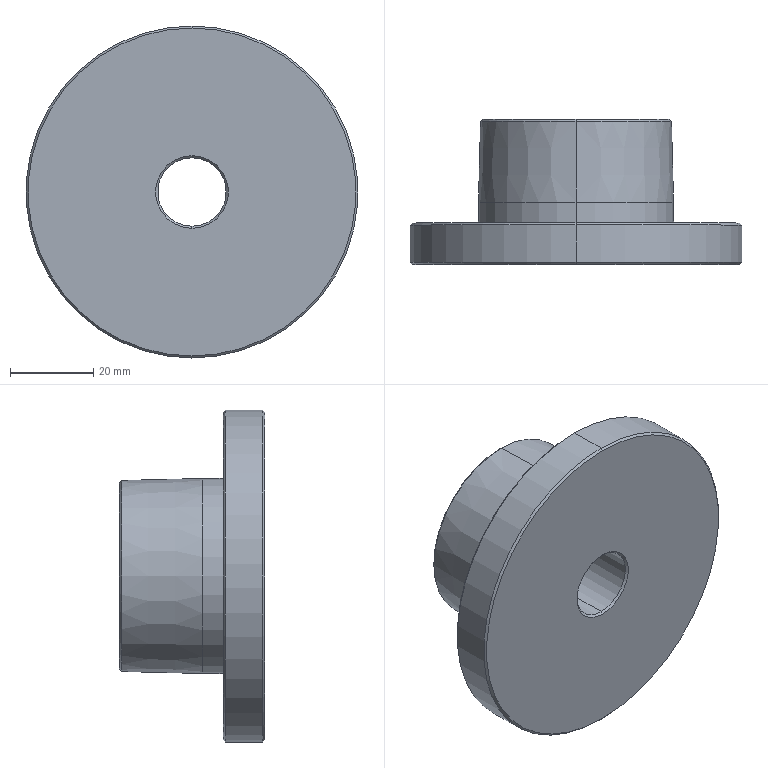Part | SolidWorks | features Chamfer 1, Revolution 1 | 1 solid | 21 faces | box 80 x 35 x 80 mm | volume 85328 mm3 | cone 12 | cylinder 6 | plane 3 | commonest cylinder face diameters 16.5 x2 47 x2 80 x2
STEP:
#1=CARTESIAN_POINT('',(0.,35.,22.5));
#2=VERTEX_POINT('',#1);
#3=CARTESIAN_POINT('',(0.,35.,-22.5));
#4=VERTEX_POINT('',#3);
#5=CARTESIAN_POINT('',(0.,35.,0.));
#6=DIRECTION('',(0.,1.,0.));
#7=DIRECTION('',(0.,0.,1.));
#8=AXIS2_PLACEMENT_3D('',#5,#6,#7);
#9=CIRCLE('',#8,22.5);
#10=EDGE_CURVE('',#2,#4,#9,.T.);
#11=ORIENTED_EDGE('',*,*,#10,.F.);
#12=CARTESIAN_POINT('',(0.,34.487,23.013));
#13=VERTEX_POINT('',#12);
#14=CARTESIAN_POINT('',(0.,34.487,23.013));
#15=DIRECTION('',(0.,-0.7071,0.7071));
#16=VECTOR('',#15,1000.);
#17=LINE('',#14,#16);
#18=EDGE_CURVE('',#2,#13,#17,.T.);
#19=ORIENTED_EDGE('',*,*,#18,.T.);
#20=CARTESIAN_POINT('',(0.,34.487,-23.013));
#21=VERTEX_POINT('',#20);
#22=CARTESIAN_POINT('',(0.,34.487,0.));
#23=DIRECTION('',(0.,-1.,0.));
#24=DIRECTION('',(0.,0.,1.));
#25=AXIS2_PLACEMENT_3D('',#22,#23,#24);
#26=CIRCLE('',#25,23.013);
#27=EDGE_CURVE('',#21,#13,#26,.T.);
#28=ORIENTED_EDGE('',*,*,#27,.F.);
#29=CARTESIAN_POINT('',(0.,34.487,-23.013));
#30=DIRECTION('',(0.,-0.7071,-0.7071));
#31=VECTOR('',#30,1000.);
#32=LINE('',#29,#31);
#33=EDGE_CURVE('',#4,#21,#32,.T.);
#34=ORIENTED_EDGE('',*,*,#33,.F.);
#35=EDGE_LOOP('',(#11,#19,#28,#34));
#36=FACE_OUTER_BOUND('',#35,.T.);
#37=CARTESIAN_POINT('',(0.,34.487,0.));
#38=DIRECTION('',(0.,-1.,0.));
#39=DIRECTION('',(0.,0.,-1.));
#40=AXIS2_PLACEMENT_3D('',#37,#38,#39);
#41=CONICAL_SURFACE('',#40,23.013,0.7854);
#42=ADVANCED_FACE('',(#36),#41,.T.);
#43=CARTESIAN_POINT('',(0.,10.,39.5));
#44=VERTEX_POINT('',#43);
#45=CARTESIAN_POINT('',(0.,10.,-39.5));
#46=VERTEX_POINT('',#45);
#47=CARTESIAN_POINT('',(0.,10.,0.));
#48=DIRECTION('',(0.,1.,0.));
#49=DIRECTION('',(0.,0.,1.));
#50=AXIS2_PLACEMENT_3D('',#47,#48,#49);
#51=CIRCLE('',#50,39.5);
#52=EDGE_CURVE('',#44,#46,#51,.T.);
#53=ORIENTED_EDGE('',*,*,#52,.F.);
#54=CARTESIAN_POINT('',(0.,9.5,40.));
#55=VERTEX_POINT('',#54);
#56=CARTESIAN_POINT('',(0.,9.5,40.));
#57=DIRECTION('',(0.,-0.7071,0.7071));
#58=VECTOR('',#57,1000.);
#59=LINE('',#56,#58);
#60=EDGE_CURVE('',#44,#55,#59,.T.);
#61=ORIENTED_EDGE('',*,*,#60,.T.);
#62=CARTESIAN_POINT('',(0.,9.5,-40.));
#63=VERTEX_POINT('',#62);
#64=CARTESIAN_POINT('',(0.,9.5,0.));
#65=DIRECTION('',(0.,-1.,0.));
#66=DIRECTION('',(0.,0.,1.));
#67=AXIS2_PLACEMENT_3D('',#64,#65,#66);
#68=CIRCLE('',#67,40.);
#69=EDGE_CURVE('',#63,#55,#68,.T.);
#70=ORIENTED_EDGE('',*,*,#69,.F.);
#71=CARTESIAN_POINT('',(0.,9.5,-40.));
#72=DIRECTION('',(0.,-0.7071,-0.7071));
#73=VECTOR('',#72,1000.);
#74=LINE('',#71,#73);
#75=EDGE_CURVE('',#46,#63,#74,.T.);
#76=ORIENTED_EDGE('',*,*,#75,.F.);
#77=EDGE_LOOP('',(#53,#61,#70,#76));
#78=FACE_OUTER_BOUND('',#77,.T.);
#79=CARTESIAN_POINT('',(0.,9.5,0.));
#80=DIRECTION('',(0.,-1.,0.));
#81=DIRECTION('',(0.,0.,-1.));
#82=AXIS2_PLACEMENT_3D('',#79,#80,#81);
#83=CONICAL_SURFACE('',#82,40.,0.7854);
#84=ADVANCED_FACE('',(#78),#83,.T.);
#85=CARTESIAN_POINT('',(0.,0.,-39.5));
#86=VERTEX_POINT('',#85);
#87=CARTESIAN_POINT('',(0.,0.,39.5));
#88=VERTEX_POINT('',#87);
#89=CARTESIAN_POINT('',(0.,0.,0.));
#90=DIRECTION('',(0.,-1.,0.));
#91=DIRECTION('',(0.,0.,-1.));
#92=AXIS2_PLACEMENT_3D('',#89,#90,#91);
#93=CIRCLE('',#92,39.5);
#94=EDGE_CURVE('',#86,#88,#93,.T.);
#95=ORIENTED_EDGE('',*,*,#94,.F.);
#96=CARTESIAN_POINT('',(0.,0.5,-40.));
#97=VERTEX_POINT('',#96);
#98=CARTESIAN_POINT('',(0.,0.,-39.5));
#99=DIRECTION('',(0.,0.7071,-0.7071));
#100=VECTOR('',#99,1000.);
#101=LINE('',#98,#100);
#102=EDGE_CURVE('',#86,#97,#101,.T.);
#103=ORIENTED_EDGE('',*,*,#102,.T.);
#104=CARTESIAN_POINT('',(0.,0.5,40.));
#105=VERTEX_POINT('',#104);
#106=CARTESIAN_POINT('',(0.,0.5,0.));
#107=DIRECTION('',(0.,1.,0.));
#108=DIRECTION('',(0.,0.,-1.));
#109=AXIS2_PLACEMENT_3D('',#106,#107,#108);
#110=CIRCLE('',#109,40.);
#111=EDGE_CURVE('',#105,#97,#110,.T.);
#112=ORIENTED_EDGE('',*,*,#111,.F.);
#113=CARTESIAN_POINT('',(0.,0.,39.5));
#114=DIRECTION('',(0.,0.7071,0.7071));
#115=VECTOR('',#114,1000.);
#116=LINE('',#113,#115);
#117=EDGE_CURVE('',#88,#105,#116,.T.);
#118=ORIENTED_EDGE('',*,*,#117,.F.);
#119=EDGE_LOOP('',(#95,#103,#112,#118));
#120=FACE_OUTER_BOUND('',#119,.T.);
#121=CARTESIAN_POINT('',(0.,0.,0.));
#122=DIRECTION('',(0.,1.,0.));
#123=DIRECTION('',(0.,0.,1.));
#124=AXIS2_PLACEMENT_3D('',#121,#122,#123);
#125=CONICAL_SURFACE('',#124,39.5,0.7854);
#126=ADVANCED_FACE('',(#120),#125,.T.);
#127=CARTESIAN_POINT('',(0.,0.5,8.25));
#128=VERTEX_POINT('',#127);
#129=CARTESIAN_POINT('',(0.,0.5,-8.25));
#130=VERTEX_POINT('',#129);
#131=CARTESIAN_POINT('',(0.,0.5,0.));
#132=DIRECTION('',(0.,-1.,0.));
#133=DIRECTION('',(0.,0.,-1.));
#134=AXIS2_PLACEMENT_3D('',#131,#132,#133);
#135=CIRCLE('',#134,8.25);
#136=EDGE_CURVE('',#128,#130,#135,.T.);
#137=ORIENTED_EDGE('',*,*,#136,.F.);
#138=CARTESIAN_POINT('',(0.,0.,8.75));
#139=VERTEX_POINT('',#138);
#140=CARTESIAN_POINT('',(0.,0.5,8.25));
#141=DIRECTION('',(0.,-0.7071,0.7071));
#142=VECTOR('',#141,1000.);
#143=LINE('',#140,#142);
#144=EDGE_CURVE('',#128,#139,#143,.T.);
#145=ORIENTED_EDGE('',*,*,#144,.T.);
#146=CARTESIAN_POINT('',(0.,0.,-8.75));
#147=VERTEX_POINT('',#146);
#148=CARTESIAN_POINT('',(0.,0.,0.));
#149=DIRECTION('',(0.,1.,0.));
#150=DIRECTION('',(0.,0.,-1.));
#151=AXIS2_PLACEMENT_3D('',#148,#149,#150);
#152=CIRCLE('',#151,8.75);
#153=EDGE_CURVE('',#147,#139,#152,.T.);
#154=ORIENTED_EDGE('',*,*,#153,.F.);
#155=CARTESIAN_POINT('',(0.,0.5,-8.25));
#156=DIRECTION('',(0.,-0.7071,-0.7071));
#157=VECTOR('',#156,1000.);
#158=LINE('',#155,#157);
#159=EDGE_CURVE('',#130,#147,#158,.T.);
#160=ORIENTED_EDGE('',*,*,#159,.F.);
#161=EDGE_LOOP('',(#137,#145,#154,#160));
#162=FACE_OUTER_BOUND('',#161,.T.);
#163=CARTESIAN_POINT('',(0.,0.5,0.));
#164=DIRECTION('',(0.,-1.,0.));
#165=DIRECTION('',(0.,0.,-1.));
#166=AXIS2_PLACEMENT_3D('',#163,#164,#165);
#167=CONICAL_SURFACE('',#166,8.25,0.7854);
#168=ADVANCED_FACE('',(#162),#167,.F.);
#169=CARTESIAN_POINT('',(0.,34.5,-8.25));
#170=VERTEX_POINT('',#169);
#171=CARTESIAN_POINT('',(0.,34.5,8.25));
#172=VERTEX_POINT('',#171);
#173=CARTESIAN_POINT('',(0.,34.5,0.));
#174=DIRECTION('',(0.,1.,0.));
#175=DIRECTION('',(0.,0.,1.));
#176=AXIS2_PLACEMENT_3D('',#173,#174,#175);
#177=CIRCLE('',#176,8.25);
#178=EDGE_CURVE('',#170,#172,#177,.T.);
#179=ORIENTED_EDGE('',*,*,#178,.F.);
#180=CARTESIAN_POINT('',(0.,35.,-8.75));
#181=VERTEX_POINT('',#180);
#182=CARTESIAN_POINT('',(0.,35.,-8.75));
#183=DIRECTION('',(0.,0.7071,-0.7071));
#184=VECTOR('',#183,1000.);
#185=LINE('',#182,#184);
#186=EDGE_CURVE('',#170,#181,#185,.T.);
#187=ORIENTED_EDGE('',*,*,#186,.T.);
#188=CARTESIAN_POINT('',(0.,35.,8.75));
#189=VERTEX_POINT('',#188);
#190=CARTESIAN_POINT('',(0.,35.,0.));
#191=DIRECTION('',(0.,-1.,0.));
#192=DIRECTION('',(0.,0.,1.));
#193=AXIS2_PLACEMENT_3D('',#190,#191,#192);
#194=CIRCLE('',#193,8.75);
#195=EDGE_CURVE('',#189,#181,#194,.T.);
#196=ORIENTED_EDGE('',*,*,#195,.F.);
#197=CARTESIAN_POINT('',(0.,35.,8.75));
#198=DIRECTION('',(0.,0.7071,0.7071));
#199=VECTOR('',#198,1000.);
#200=LINE('',#197,#199);
#201=EDGE_CURVE('',#172,#189,#200,.T.);
#202=ORIENTED_EDGE('',*,*,#201,.F.);
#203=EDGE_LOOP('',(#179,#187,#196,#202));
#204=FACE_OUTER_BOUND('',#203,.T.);
#205=CARTESIAN_POINT('',(0.,35.,0.));
#206=DIRECTION('',(0.,1.,0.));
#207=DIRECTION('',(0.,0.,1.));
#208=AXIS2_PLACEMENT_3D('',#205,#206,#207);
#209=CONICAL_SURFACE('',#208,8.75,0.7854);
#210=ADVANCED_FACE('',(#204),#209,.F.);
#211=CARTESIAN_POINT('',(0.,15.,-23.5));
#212=VERTEX_POINT('',#211);
#213=CARTESIAN_POINT('',(0.,15.,23.5));
#214=VERTEX_POINT('',#213);
#215=CARTESIAN_POINT('',(0.,15.,0.));
#216=DIRECTION('',(0.,-1.,0.));
#217=DIRECTION('',(0.,0.,-1.));
#218=AXIS2_PLACEMENT_3D('',#215,#216,#217);
#219=CIRCLE('',#218,23.5);
#220=EDGE_CURVE('',#212,#214,#219,.T.);
#221=ORIENTED_EDGE('',*,*,#220,.T.);
#222=CARTESIAN_POINT('',(0.,10.,23.5));
#223=VERTEX_POINT('',#222);
#224=CARTESIAN_POINT('',(0.,0.,23.5));
#225=DIRECTION('',(0.,-1.,0.));
#226=VECTOR('',#225,1000.);
#227=LINE('',#224,#226);
#228=EDGE_CURVE('',#214,#223,#227,.T.);
#229=ORIENTED_EDGE('',*,*,#228,.T.);
#230=CARTESIAN_POINT('',(0.,10.,-23.5));
#231=VERTEX_POINT('',#230);
#232=CARTESIAN_POINT('',(0.,10.,0.));
#233=DIRECTION('',(0.,-1.,0.));
#234=DIRECTION('',(0.,0.,-1.));
#235=AXIS2_PLACEMENT_3D('',#232,#233,#234);
#236=CIRCLE('',#235,23.5);
#237=EDGE_CURVE('',#231,#223,#236,.T.);
#238=ORIENTED_EDGE('',*,*,#237,.F.);
#239=CARTESIAN_POINT('',(0.,0.,-23.5));
#240=DIRECTION('',(0.,-1.,0.));
#241=VECTOR('',#240,1000.);
#242=LINE('',#239,#241);
#243=EDGE_CURVE('',#212,#231,#242,.T.);
#244=ORIENTED_EDGE('',*,*,#243,.F.);
#245=EDGE_LOOP('',(#221,#229,#238,#244));
#246=FACE_OUTER_BOUND('',#245,.T.);
#247=CARTESIAN_POINT('',(0.,0.,0.));
#248=DIRECTION('',(0.,-1.,0.));
#249=DIRECTION('',(0.,0.,-1.));
#250=AXIS2_PLACEMENT_3D('',#247,#248,#249);
#251=CYLINDRICAL_SURFACE('',#250,23.5);
#252=ADVANCED_FACE('',(#246),#251,.T.);
#253=ORIENTED_EDGE('',*,*,#69,.T.);
#254=CARTESIAN_POINT('',(0.,0.,40.));
#255=DIRECTION('',(0.,-1.,0.));
#256=VECTOR('',#255,1000.);
#257=LINE('',#254,#256);
#258=EDGE_CURVE('',#55,#105,#257,.T.);
#259=ORIENTED_EDGE('',*,*,#258,.T.);
#260=ORIENTED_EDGE('',*,*,#111,.T.);
#261=CARTESIAN_POINT('',(0.,0.,-40.));
#262=DIRECTION('',(0.,-1.,0.));
#263=VECTOR('',#262,1000.);
#264=LINE('',#261,#263);
#265=EDGE_CURVE('',#63,#97,#264,.T.);
#266=ORIENTED_EDGE('',*,*,#265,.F.);
#267=EDGE_LOOP('',(#253,#259,#260,#266));
#268=FACE_OUTER_BOUND('',#267,.T.);
#269=CARTESIAN_POINT('',(0.,0.,0.));
#270=DIRECTION('',(0.,-1.,0.));
#271=DIRECTION('',(0.,0.,-1.));
#272=AXIS2_PLACEMENT_3D('',#269,#270,#271);
#273=CYLINDRICAL_SURFACE('',#272,40.);
#274=ADVANCED_FACE('',(#268),#273,.T.);
#275=ORIENTED_EDGE('',*,*,#178,.T.);
#276=CARTESIAN_POINT('',(0.,0.,8.25));
#277=DIRECTION('',(0.,-1.,0.));
#278=VECTOR('',#277,1000.);
#279=LINE('',#276,#278);
#280=EDGE_CURVE('',#172,#128,#279,.T.);
#281=ORIENTED_EDGE('',*,*,#280,.T.);
#282=ORIENTED_EDGE('',*,*,#136,.T.);
#283=CARTESIAN_POINT('',(0.,0.,-8.25));
#284=DIRECTION('',(0.,-1.,0.));
#285=VECTOR('',#284,1000.);
#286=LINE('',#283,#285);
#287=EDGE_CURVE('',#170,#130,#286,.T.);
#288=ORIENTED_EDGE('',*,*,#287,.F.);
#289=EDGE_LOOP('',(#275,#281,#282,#288));
#290=FACE_OUTER_BOUND('',#289,.T.);
#291=CARTESIAN_POINT('',(0.,0.,0.));
#292=DIRECTION('',(0.,-1.,0.));
#293=DIRECTION('',(0.,0.,-1.));
#294=AXIS2_PLACEMENT_3D('',#291,#292,#293);
#295=CYLINDRICAL_SURFACE('',#294,8.25);
#296=ADVANCED_FACE('',(#290),#295,.F.);
#297=ORIENTED_EDGE('',*,*,#27,.T.);
#298=CARTESIAN_POINT('',(0.,15.,23.5));
#299=DIRECTION('',(0.,-0.9997,0.02499));
#300=VECTOR('',#299,1000.);
#301=LINE('',#298,#300);
#302=EDGE_CURVE('',#13,#214,#301,.T.);
#303=ORIENTED_EDGE('',*,*,#302,.T.);
#304=ORIENTED_EDGE('',*,*,#220,.F.);
#305=CARTESIAN_POINT('',(0.,15.,-23.5));
#306=DIRECTION('',(0.,-0.9997,-0.02499));
#307=VECTOR('',#306,1000.);
#308=LINE('',#305,#307);
#309=EDGE_CURVE('',#21,#212,#308,.T.);
#310=ORIENTED_EDGE('',*,*,#309,.F.);
#311=EDGE_LOOP('',(#297,#303,#304,#310));
#312=FACE_OUTER_BOUND('',#311,.T.);
#313=CARTESIAN_POINT('',(0.,15.,0.));
#314=DIRECTION('',(0.,-1.,0.));
#315=DIRECTION('',(0.,0.,-1.));
#316=AXIS2_PLACEMENT_3D('',#313,#314,#315);
#317=CONICAL_SURFACE('',#316,23.5,0.02499);
#318=ADVANCED_FACE('',(#312),#317,.T.);
#319=ORIENTED_EDGE('',*,*,#302,.F.);
#320=CARTESIAN_POINT('',(0.,34.487,0.));
#321=DIRECTION('',(0.,-1.,0.));
#322=DIRECTION('',(0.,0.,1.));
#323=AXIS2_PLACEMENT_3D('',#320,#321,#322);
#324=CIRCLE('',#323,23.013);
#325=EDGE_CURVE('',#13,#21,#324,.T.);
#326=ORIENTED_EDGE('',*,*,#325,.T.);
#327=ORIENTED_EDGE('',*,*,#309,.T.);
#328=CARTESIAN_POINT('',(0.,15.,0.));
#329=DIRECTION('',(0.,-1.,0.));
#330=DIRECTION('',(0.,0.,-1.));
#331=AXIS2_PLACEMENT_3D('',#328,#329,#330);
#332=CIRCLE('',#331,23.5);
#333=EDGE_CURVE('',#214,#212,#332,.T.);
#334=ORIENTED_EDGE('',*,*,#333,.F.);
#335=EDGE_LOOP('',(#319,#326,#327,#334));
#336=FACE_OUTER_BOUND('',#335,.T.);
#337=CARTESIAN_POINT('',(0.,15.,0.));
#338=DIRECTION('',(0.,-1.,0.));
#339=DIRECTION('',(0.,0.,-1.));
#340=AXIS2_PLACEMENT_3D('',#337,#338,#339);
#341=CONICAL_SURFACE('',#340,23.5,0.02499);
#342=ADVANCED_FACE('',(#336),#341,.T.);
#343=ORIENTED_EDGE('',*,*,#195,.T.);
#344=CARTESIAN_POINT('',(0.,35.,0.));
#345=DIRECTION('',(0.,-1.,0.));
#346=DIRECTION('',(0.,0.,1.));
#347=AXIS2_PLACEMENT_3D('',#344,#345,#346);
#348=CIRCLE('',#347,8.75);
#349=EDGE_CURVE('',#181,#189,#348,.T.);
#350=ORIENTED_EDGE('',*,*,#349,.T.);
#351=EDGE_LOOP('',(#343,#350));
#352=FACE_BOUND('',#351,.T.);
#353=CARTESIAN_POINT('',(0.,35.,0.));
#354=DIRECTION('',(0.,1.,0.));
#355=DIRECTION('',(0.,0.,1.));
#356=AXIS2_PLACEMENT_3D('',#353,#354,#355);
#357=CIRCLE('',#356,22.5);
#358=EDGE_CURVE('',#4,#2,#357,.T.);
#359=ORIENTED_EDGE('',*,*,#358,.T.);
#360=ORIENTED_EDGE('',*,*,#10,.T.);
#361=EDGE_LOOP('',(#359,#360));
#362=FACE_OUTER_BOUND('',#361,.T.);
#363=CARTESIAN_POINT('',(8.25,35.,0.));
#364=DIRECTION('',(0.,1.,0.));
#365=DIRECTION('',(0.,0.,1.));
#366=AXIS2_PLACEMENT_3D('',#363,#364,#365);
#367=PLANE('',#366);
#368=ADVANCED_FACE('',(#352,#362),#367,.T.);
#369=ORIENTED_EDGE('',*,*,#280,.F.);
#370=CARTESIAN_POINT('',(0.,34.5,0.));
#371=DIRECTION('',(0.,1.,0.));
#372=DIRECTION('',(0.,0.,1.));
#373=AXIS2_PLACEMENT_3D('',#370,#371,#372);
#374=CIRCLE('',#373,8.25);
#375=EDGE_CURVE('',#172,#170,#374,.T.);
#376=ORIENTED_EDGE('',*,*,#375,.T.);
#377=ORIENTED_EDGE('',*,*,#287,.T.);
#378=CARTESIAN_POINT('',(0.,0.5,0.));
#379=DIRECTION('',(0.,-1.,0.));
#380=DIRECTION('',(0.,0.,-1.));
#381=AXIS2_PLACEMENT_3D('',#378,#379,#380);
#382=CIRCLE('',#381,8.25);
#383=EDGE_CURVE('',#130,#128,#382,.T.);
#384=ORIENTED_EDGE('',*,*,#383,.T.);
#385=EDGE_LOOP('',(#369,#376,#377,#384));
#386=FACE_OUTER_BOUND('',#385,.T.);
#387=CARTESIAN_POINT('',(0.,0.,0.));
#388=DIRECTION('',(0.,-1.,0.));
#389=DIRECTION('',(0.,0.,-1.));
#390=AXIS2_PLACEMENT_3D('',#387,#388,#389);
#391=CYLINDRICAL_SURFACE('',#390,8.25);
#392=ADVANCED_FACE('',(#386),#391,.F.);
#393=ORIENTED_EDGE('',*,*,#153,.T.);
#394=CARTESIAN_POINT('',(0.,0.,0.));
#395=DIRECTION('',(0.,1.,0.));
#396=DIRECTION('',(0.,0.,-1.));
#397=AXIS2_PLACEMENT_3D('',#394,#395,#396);
#398=CIRCLE('',#397,8.75);
#399=EDGE_CURVE('',#139,#147,#398,.T.);
#400=ORIENTED_EDGE('',*,*,#399,.T.);
#401=EDGE_LOOP('',(#393,#400));
#402=FACE_BOUND('',#401,.T.);
#403=CARTESIAN_POINT('',(0.,0.,0.));
#404=DIRECTION('',(0.,-1.,0.));
#405=DIRECTION('',(0.,0.,-1.));
#406=AXIS2_PLACEMENT_3D('',#403,#404,#405);
#407=CIRCLE('',#406,39.5);
#408=EDGE_CURVE('',#88,#86,#407,.T.);
#409=ORIENTED_EDGE('',*,*,#408,.T.);
#410=ORIENTED_EDGE('',*,*,#94,.T.);
#411=EDGE_LOOP('',(#409,#410));
#412=FACE_OUTER_BOUND('',#411,.T.);
#413=CARTESIAN_POINT('',(40.,0.,0.));
#414=DIRECTION('',(0.,-1.,0.));
#415=DIRECTION('',(0.,0.,-1.));
#416=AXIS2_PLACEMENT_3D('',#413,#414,#415);
#417=PLANE('',#416);
#418=ADVANCED_FACE('',(#402,#412),#417,.T.);
#419=ORIENTED_EDGE('',*,*,#258,.F.);
#420=CARTESIAN_POINT('',(0.,9.5,0.));
#421=DIRECTION('',(0.,-1.,0.));
#422=DIRECTION('',(0.,0.,1.));
#423=AXIS2_PLACEMENT_3D('',#420,#421,#422);
#424=CIRCLE('',#423,40.);
#425=EDGE_CURVE('',#55,#63,#424,.T.);
#426=ORIENTED_EDGE('',*,*,#425,.T.);
#427=ORIENTED_EDGE('',*,*,#265,.T.);
#428=CARTESIAN_POINT('',(0.,0.5,0.));
#429=DIRECTION('',(0.,1.,0.));
#430=DIRECTION('',(0.,0.,-1.));
#431=AXIS2_PLACEMENT_3D('',#428,#429,#430);
#432=CIRCLE('',#431,40.);
#433=EDGE_CURVE('',#97,#105,#432,.T.);
#434=ORIENTED_EDGE('',*,*,#433,.T.);
#435=EDGE_LOOP('',(#419,#426,#427,#434));
#436=FACE_OUTER_BOUND('',#435,.T.);
#437=CARTESIAN_POINT('',(0.,0.,0.));
#438=DIRECTION('',(0.,-1.,0.));
#439=DIRECTION('',(0.,0.,-1.));
#440=AXIS2_PLACEMENT_3D('',#437,#438,#439);
#441=CYLINDRICAL_SURFACE('',#440,40.);
#442=ADVANCED_FACE('',(#436),#441,.T.);
#443=CARTESIAN_POINT('',(0.,10.,0.));
#444=DIRECTION('',(0.,1.,0.));
#445=DIRECTION('',(0.,0.,1.));
#446=AXIS2_PLACEMENT_3D('',#443,#444,#445);
#447=CIRCLE('',#446,39.5);
#448=EDGE_CURVE('',#46,#44,#447,.T.);
#449=ORIENTED_EDGE('',*,*,#448,.T.);
#450=ORIENTED_EDGE('',*,*,#52,.T.);
#451=EDGE_LOOP('',(#449,#450));
#452=FACE_OUTER_BOUND('',#451,.T.);
#453=ORIENTED_EDGE('',*,*,#237,.T.);
#454=CARTESIAN_POINT('',(0.,10.,0.));
#455=DIRECTION('',(0.,-1.,0.));
#456=DIRECTION('',(0.,0.,-1.));
#457=AXIS2_PLACEMENT_3D('',#454,#455,#456);
#458=CIRCLE('',#457,23.5);
#459=EDGE_CURVE('',#223,#231,#458,.T.);
#460=ORIENTED_EDGE('',*,*,#459,.T.);
#461=EDGE_LOOP('',(#453,#460));
#462=FACE_BOUND('',#461,.T.);
#463=CARTESIAN_POINT('',(23.5,10.,0.));
#464=DIRECTION('',(0.,1.,0.));
#465=DIRECTION('',(0.,0.,1.));
#466=AXIS2_PLACEMENT_3D('',#463,#464,#465);
#467=PLANE('',#466);
#468=ADVANCED_FACE('',(#452,#462),#467,.T.);
#469=ORIENTED_EDGE('',*,*,#228,.F.);
#470=ORIENTED_EDGE('',*,*,#333,.T.);
#471=ORIENTED_EDGE('',*,*,#243,.T.);
#472=ORIENTED_EDGE('',*,*,#459,.F.);
#473=EDGE_LOOP('',(#469,#470,#471,#472));
#474=FACE_OUTER_BOUND('',#473,.T.);
#475=CARTESIAN_POINT('',(0.,0.,0.));
#476=DIRECTION('',(0.,-1.,0.));
#477=DIRECTION('',(0.,0.,-1.));
#478=AXIS2_PLACEMENT_3D('',#475,#476,#477);
#479=CYLINDRICAL_SURFACE('',#478,23.5);
#480=ADVANCED_FACE('',(#474),#479,.T.);
#481=ORIENTED_EDGE('',*,*,#186,.F.);
#482=ORIENTED_EDGE('',*,*,#375,.F.);
#483=ORIENTED_EDGE('',*,*,#201,.T.);
#484=ORIENTED_EDGE('',*,*,#349,.F.);
#485=EDGE_LOOP('',(#481,#482,#483,#484));
#486=FACE_OUTER_BOUND('',#485,.T.);
#487=CARTESIAN_POINT('',(0.,35.,0.));
#488=DIRECTION('',(0.,1.,0.));
#489=DIRECTION('',(0.,0.,1.));
#490=AXIS2_PLACEMENT_3D('',#487,#488,#489);
#491=CONICAL_SURFACE('',#490,8.75,0.7854);
#492=ADVANCED_FACE('',(#486),#491,.F.);
#493=ORIENTED_EDGE('',*,*,#144,.F.);
#494=ORIENTED_EDGE('',*,*,#383,.F.);
#495=ORIENTED_EDGE('',*,*,#159,.T.);
#496=ORIENTED_EDGE('',*,*,#399,.F.);
#497=EDGE_LOOP('',(#493,#494,#495,#496));
#498=FACE_OUTER_BOUND('',#497,.T.);
#499=CARTESIAN_POINT('',(0.,0.5,0.));
#500=DIRECTION('',(0.,-1.,0.));
#501=DIRECTION('',(0.,0.,-1.));
#502=AXIS2_PLACEMENT_3D('',#499,#500,#501);
#503=CONICAL_SURFACE('',#502,8.25,0.7854);
#504=ADVANCED_FACE('',(#498),#503,.F.);
#505=ORIENTED_EDGE('',*,*,#102,.F.);
#506=ORIENTED_EDGE('',*,*,#408,.F.);
#507=ORIENTED_EDGE('',*,*,#117,.T.);
#508=ORIENTED_EDGE('',*,*,#433,.F.);
#509=EDGE_LOOP('',(#505,#506,#507,#508));
#510=FACE_OUTER_BOUND('',#509,.T.);
#511=CARTESIAN_POINT('',(0.,0.,0.));
#512=DIRECTION('',(0.,1.,0.));
#513=DIRECTION('',(0.,0.,1.));
#514=AXIS2_PLACEMENT_3D('',#511,#512,#513);
#515=CONICAL_SURFACE('',#514,39.5,0.7854);
#516=ADVANCED_FACE('',(#510),#515,.T.);
#517=ORIENTED_EDGE('',*,*,#60,.F.);
#518=ORIENTED_EDGE('',*,*,#448,.F.);
#519=ORIENTED_EDGE('',*,*,#75,.T.);
#520=ORIENTED_EDGE('',*,*,#425,.F.);
#521=EDGE_LOOP('',(#517,#518,#519,#520));
#522=FACE_OUTER_BOUND('',#521,.T.);
#523=CARTESIAN_POINT('',(0.,9.5,0.));
#524=DIRECTION('',(0.,-1.,0.));
#525=DIRECTION('',(0.,0.,-1.));
#526=AXIS2_PLACEMENT_3D('',#523,#524,#525);
#527=CONICAL_SURFACE('',#526,40.,0.7854);
#528=ADVANCED_FACE('',(#522),#527,.T.);
#529=ORIENTED_EDGE('',*,*,#18,.F.);
#530=ORIENTED_EDGE('',*,*,#358,.F.);
#531=ORIENTED_EDGE('',*,*,#33,.T.);
#532=ORIENTED_EDGE('',*,*,#325,.F.);
#533=EDGE_LOOP('',(#529,#530,#531,#532));
#534=FACE_OUTER_BOUND('',#533,.T.);
#535=CARTESIAN_POINT('',(0.,34.487,0.));
#536=DIRECTION('',(0.,-1.,0.));
#537=DIRECTION('',(0.,0.,-1.));
#538=AXIS2_PLACEMENT_3D('',#535,#536,#537);
#539=CONICAL_SURFACE('',#538,23.013,0.7854);
#540=ADVANCED_FACE('',(#534),#539,.T.);
#541=CLOSED_SHELL('',(#42,#84,#126,#168,#210,#252,#274,#296,#318,#342,#368,#392,#418,#442,#468,#480,#492,#504,#516,#528,#540));
#542=MANIFOLD_SOLID_BREP('',#541);
#543=CARTESIAN_POINT('',(0.,0.,0.));
#544=DIRECTION('',(0.,0.,1.));
#545=DIRECTION('',(1.,0.,0.));
#546=AXIS2_PLACEMENT_3D('',#543,#544,#545);
#547=(LENGTH_UNIT()NAMED_UNIT(*)SI_UNIT(.MILLI.,.METRE.));
#548=UNCERTAINTY_MEASURE_WITH_UNIT(LENGTH_MEASURE(0.00001),#547,'','');
#549=(NAMED_UNIT(*)PLANE_ANGLE_UNIT()SI_UNIT($,.RADIAN.));
#550=(NAMED_UNIT(*)SI_UNIT($,.STERADIAN.)SOLID_ANGLE_UNIT());
#551=(GEOMETRIC_REPRESENTATION_CONTEXT(3)GLOBAL_UNCERTAINTY_ASSIGNED_CONTEXT((#548))GLOBAL_UNIT_ASSIGNED_CONTEXT((#547,#549,#550))REPRESENTATION_CONTEXT('',''));
#552=ADVANCED_BREP_SHAPE_REPRESENTATION('',(#542,#546),#551);